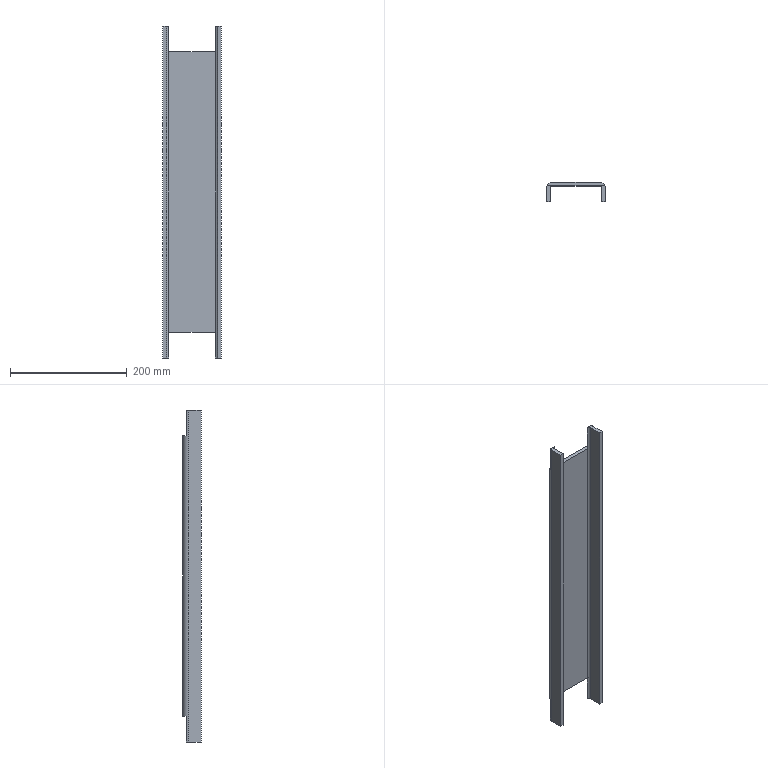Part | SolidWorks | features ICE 2, Extrusion 1 | 1 solid | 22 faces | box 100 x 32 x 568 mm | volume 448322 mm3 | plane 18 | cylinder 4 | commonest cylinder face diameters 8 x2 20 x2
STEP:
#1=CARTESIAN_POINT('',(90.,32.,524.));
#2=VERTEX_POINT('',#1);
#3=CARTESIAN_POINT('',(90.,32.,44.));
#4=VERTEX_POINT('',#3);
#5=CARTESIAN_POINT('',(90.,32.,568.));
#6=DIRECTION('',(0.,0.,-1.));
#7=VECTOR('',#6,1000.);
#8=LINE('',#5,#7);
#9=EDGE_CURVE('',#2,#4,#8,.T.);
#10=ORIENTED_EDGE('',*,*,#9,.T.);
#11=CARTESIAN_POINT('',(10.,32.,44.));
#12=VERTEX_POINT('',#11);
#13=CARTESIAN_POINT('',(10.,32.,44.));
#14=DIRECTION('',(-1.,0.,0.));
#15=VECTOR('',#14,1000.);
#16=LINE('',#13,#15);
#17=EDGE_CURVE('',#4,#12,#16,.T.);
#18=ORIENTED_EDGE('',*,*,#17,.T.);
#19=CARTESIAN_POINT('',(10.,32.,524.));
#20=VERTEX_POINT('',#19);
#21=CARTESIAN_POINT('',(10.,32.,568.));
#22=DIRECTION('',(0.,0.,-1.));
#23=VECTOR('',#22,1000.);
#24=LINE('',#21,#23);
#25=EDGE_CURVE('',#20,#12,#24,.T.);
#26=ORIENTED_EDGE('',*,*,#25,.F.);
#27=CARTESIAN_POINT('',(10.,32.,524.));
#28=DIRECTION('',(1.,0.,0.));
#29=VECTOR('',#28,1000.);
#30=LINE('',#27,#29);
#31=EDGE_CURVE('',#20,#2,#30,.T.);
#32=ORIENTED_EDGE('',*,*,#31,.T.);
#33=EDGE_LOOP('',(#10,#18,#26,#32));
#34=FACE_OUTER_BOUND('',#33,.T.);
#35=CARTESIAN_POINT('',(10.,32.,568.));
#36=DIRECTION('',(0.,1.,0.));
#37=DIRECTION('',(0.,0.,1.));
#38=AXIS2_PLACEMENT_3D('',#35,#36,#37);
#39=PLANE('',#38);
#40=ADVANCED_FACE('',(#34),#39,.T.);
#41=CARTESIAN_POINT('',(90.,26.,44.));
#42=VERTEX_POINT('',#41);
#43=CARTESIAN_POINT('',(10.,26.,44.));
#44=VERTEX_POINT('',#43);
#45=CARTESIAN_POINT('',(112.02,26.,44.));
#46=DIRECTION('',(-1.,0.,0.));
#47=VECTOR('',#46,1000.);
#48=LINE('',#45,#47);
#49=EDGE_CURVE('',#42,#44,#48,.T.);
#50=ORIENTED_EDGE('',*,*,#49,.F.);
#51=CARTESIAN_POINT('',(90.,26.,524.));
#52=VERTEX_POINT('',#51);
#53=CARTESIAN_POINT('',(90.,26.,568.));
#54=DIRECTION('',(0.,0.,-1.));
#55=VECTOR('',#54,1000.);
#56=LINE('',#53,#55);
#57=EDGE_CURVE('',#52,#42,#56,.T.);
#58=ORIENTED_EDGE('',*,*,#57,.F.);
#59=CARTESIAN_POINT('',(10.,26.,524.));
#60=VERTEX_POINT('',#59);
#61=CARTESIAN_POINT('',(-5.017,26.,524.));
#62=DIRECTION('',(1.,0.,0.));
#63=VECTOR('',#62,1000.);
#64=LINE('',#61,#63);
#65=EDGE_CURVE('',#60,#52,#64,.T.);
#66=ORIENTED_EDGE('',*,*,#65,.F.);
#67=CARTESIAN_POINT('',(10.,26.,568.));
#68=DIRECTION('',(0.,0.,-1.));
#69=VECTOR('',#68,1000.);
#70=LINE('',#67,#69);
#71=EDGE_CURVE('',#60,#44,#70,.T.);
#72=ORIENTED_EDGE('',*,*,#71,.T.);
#73=EDGE_LOOP('',(#50,#58,#66,#72));
#74=FACE_OUTER_BOUND('',#73,.T.);
#75=CARTESIAN_POINT('',(10.,26.,568.));
#76=DIRECTION('',(0.,1.,0.));
#77=DIRECTION('',(0.,0.,1.));
#78=AXIS2_PLACEMENT_3D('',#75,#76,#77);
#79=PLANE('',#78);
#80=ADVANCED_FACE('',(#74),#79,.F.);
#81=CARTESIAN_POINT('',(99.165,26.,0.));
#82=VERTEX_POINT('',#81);
#83=CARTESIAN_POINT('',(90.,26.,0.));
#84=VERTEX_POINT('',#83);
#85=CARTESIAN_POINT('',(90.,26.,0.));
#86=DIRECTION('',(-1.,0.,0.));
#87=VECTOR('',#86,1000.);
#88=LINE('',#85,#87);
#89=EDGE_CURVE('',#82,#84,#88,.T.);
#90=ORIENTED_EDGE('',*,*,#89,.F.);
#91=CARTESIAN_POINT('',(100.,22.,0.));
#92=VERTEX_POINT('',#91);
#93=CARTESIAN_POINT('',(90.,22.,0.));
#94=DIRECTION('',(0.,0.,-1.));
#95=DIRECTION('',(-1.,0.,0.));
#96=AXIS2_PLACEMENT_3D('',#93,#94,#95);
#97=CIRCLE('',#96,10.);
#98=EDGE_CURVE('',#82,#92,#97,.T.);
#99=ORIENTED_EDGE('',*,*,#98,.T.);
#100=CARTESIAN_POINT('',(100.,0.,0.));
#101=VERTEX_POINT('',#100);
#102=CARTESIAN_POINT('',(100.,22.,0.));
#103=DIRECTION('',(0.,-1.,0.));
#104=VECTOR('',#103,1000.);
#105=LINE('',#102,#104);
#106=EDGE_CURVE('',#92,#101,#105,.T.);
#107=ORIENTED_EDGE('',*,*,#106,.T.);
#108=CARTESIAN_POINT('',(94.,0.,0.));
#109=VERTEX_POINT('',#108);
#110=CARTESIAN_POINT('',(94.,0.,0.));
#111=DIRECTION('',(1.,0.,0.));
#112=VECTOR('',#111,1000.);
#113=LINE('',#110,#112);
#114=EDGE_CURVE('',#109,#101,#113,.T.);
#115=ORIENTED_EDGE('',*,*,#114,.F.);
#116=CARTESIAN_POINT('',(94.,22.,0.));
#117=VERTEX_POINT('',#116);
#118=CARTESIAN_POINT('',(94.,22.,0.));
#119=DIRECTION('',(0.,-1.,0.));
#120=VECTOR('',#119,1000.);
#121=LINE('',#118,#120);
#122=EDGE_CURVE('',#117,#109,#121,.T.);
#123=ORIENTED_EDGE('',*,*,#122,.F.);
#124=CARTESIAN_POINT('',(90.,22.,0.));
#125=DIRECTION('',(0.,0.,-1.));
#126=DIRECTION('',(-1.,0.,0.));
#127=AXIS2_PLACEMENT_3D('',#124,#125,#126);
#128=CIRCLE('',#127,4.);
#129=EDGE_CURVE('',#84,#117,#128,.T.);
#130=ORIENTED_EDGE('',*,*,#129,.F.);
#131=EDGE_LOOP('',(#90,#99,#107,#115,#123,#130));
#132=FACE_OUTER_BOUND('',#131,.T.);
#133=CARTESIAN_POINT('',(90.,22.,0.));
#134=DIRECTION('',(0.,0.,-1.));
#135=DIRECTION('',(-1.,0.,0.));
#136=AXIS2_PLACEMENT_3D('',#133,#134,#135);
#137=PLANE('',#136);
#138=ADVANCED_FACE('',(#132),#137,.T.);
#139=CARTESIAN_POINT('',(99.165,26.,568.));
#140=VERTEX_POINT('',#139);
#141=CARTESIAN_POINT('',(100.,22.,568.));
#142=VERTEX_POINT('',#141);
#143=CARTESIAN_POINT('',(90.,22.,568.));
#144=DIRECTION('',(0.,0.,-1.));
#145=DIRECTION('',(-1.,0.,0.));
#146=AXIS2_PLACEMENT_3D('',#143,#144,#145);
#147=CIRCLE('',#146,10.);
#148=EDGE_CURVE('',#140,#142,#147,.T.);
#149=ORIENTED_EDGE('',*,*,#148,.F.);
#150=CARTESIAN_POINT('',(90.,26.,568.));
#151=VERTEX_POINT('',#150);
#152=CARTESIAN_POINT('',(90.,26.,568.));
#153=DIRECTION('',(-1.,0.,0.));
#154=VECTOR('',#153,1000.);
#155=LINE('',#152,#154);
#156=EDGE_CURVE('',#140,#151,#155,.T.);
#157=ORIENTED_EDGE('',*,*,#156,.T.);
#158=CARTESIAN_POINT('',(94.,22.,568.));
#159=VERTEX_POINT('',#158);
#160=CARTESIAN_POINT('',(90.,22.,568.));
#161=DIRECTION('',(0.,0.,-1.));
#162=DIRECTION('',(-1.,0.,0.));
#163=AXIS2_PLACEMENT_3D('',#160,#161,#162);
#164=CIRCLE('',#163,4.);
#165=EDGE_CURVE('',#151,#159,#164,.T.);
#166=ORIENTED_EDGE('',*,*,#165,.T.);
#167=CARTESIAN_POINT('',(94.,0.,568.));
#168=VERTEX_POINT('',#167);
#169=CARTESIAN_POINT('',(94.,22.,568.));
#170=DIRECTION('',(0.,-1.,0.));
#171=VECTOR('',#170,1000.);
#172=LINE('',#169,#171);
#173=EDGE_CURVE('',#159,#168,#172,.T.);
#174=ORIENTED_EDGE('',*,*,#173,.T.);
#175=CARTESIAN_POINT('',(100.,0.,568.));
#176=VERTEX_POINT('',#175);
#177=CARTESIAN_POINT('',(94.,0.,568.));
#178=DIRECTION('',(1.,0.,0.));
#179=VECTOR('',#178,1000.);
#180=LINE('',#177,#179);
#181=EDGE_CURVE('',#168,#176,#180,.T.);
#182=ORIENTED_EDGE('',*,*,#181,.T.);
#183=CARTESIAN_POINT('',(100.,22.,568.));
#184=DIRECTION('',(0.,-1.,0.));
#185=VECTOR('',#184,1000.);
#186=LINE('',#183,#185);
#187=EDGE_CURVE('',#142,#176,#186,.T.);
#188=ORIENTED_EDGE('',*,*,#187,.F.);
#189=EDGE_LOOP('',(#149,#157,#166,#174,#182,#188));
#190=FACE_OUTER_BOUND('',#189,.T.);
#191=CARTESIAN_POINT('',(90.,22.,568.));
#192=DIRECTION('',(0.,0.,-1.));
#193=DIRECTION('',(-1.,0.,0.));
#194=AXIS2_PLACEMENT_3D('',#191,#192,#193);
#195=PLANE('',#194);
#196=ADVANCED_FACE('',(#190),#195,.F.);
#197=ORIENTED_EDGE('',*,*,#122,.T.);
#198=CARTESIAN_POINT('',(94.,0.,568.));
#199=DIRECTION('',(0.,0.,-1.));
#200=VECTOR('',#199,1000.);
#201=LINE('',#198,#200);
#202=EDGE_CURVE('',#168,#109,#201,.T.);
#203=ORIENTED_EDGE('',*,*,#202,.F.);
#204=ORIENTED_EDGE('',*,*,#173,.F.);
#205=CARTESIAN_POINT('',(94.,22.,568.));
#206=DIRECTION('',(0.,0.,-1.));
#207=VECTOR('',#206,1000.);
#208=LINE('',#205,#207);
#209=EDGE_CURVE('',#159,#117,#208,.T.);
#210=ORIENTED_EDGE('',*,*,#209,.T.);
#211=EDGE_LOOP('',(#197,#203,#204,#210));
#212=FACE_OUTER_BOUND('',#211,.T.);
#213=CARTESIAN_POINT('',(94.,22.,568.));
#214=DIRECTION('',(1.,0.,0.));
#215=DIRECTION('',(0.,0.,-1.));
#216=AXIS2_PLACEMENT_3D('',#213,#214,#215);
#217=PLANE('',#216);
#218=ADVANCED_FACE('',(#212),#217,.F.);
#219=ORIENTED_EDGE('',*,*,#114,.T.);
#220=CARTESIAN_POINT('',(100.,0.,568.));
#221=DIRECTION('',(0.,0.,-1.));
#222=VECTOR('',#221,1000.);
#223=LINE('',#220,#222);
#224=EDGE_CURVE('',#176,#101,#223,.T.);
#225=ORIENTED_EDGE('',*,*,#224,.F.);
#226=ORIENTED_EDGE('',*,*,#181,.F.);
#227=ORIENTED_EDGE('',*,*,#202,.T.);
#228=EDGE_LOOP('',(#219,#225,#226,#227));
#229=FACE_OUTER_BOUND('',#228,.T.);
#230=CARTESIAN_POINT('',(94.,0.,568.));
#231=DIRECTION('',(0.,1.,0.));
#232=DIRECTION('',(0.,0.,1.));
#233=AXIS2_PLACEMENT_3D('',#230,#231,#232);
#234=PLANE('',#233);
#235=ADVANCED_FACE('',(#229),#234,.F.);
#236=ORIENTED_EDGE('',*,*,#106,.F.);
#237=CARTESIAN_POINT('',(100.,22.,568.));
#238=DIRECTION('',(0.,0.,-1.));
#239=VECTOR('',#238,1000.);
#240=LINE('',#237,#239);
#241=EDGE_CURVE('',#142,#92,#240,.T.);
#242=ORIENTED_EDGE('',*,*,#241,.F.);
#243=ORIENTED_EDGE('',*,*,#187,.T.);
#244=ORIENTED_EDGE('',*,*,#224,.T.);
#245=EDGE_LOOP('',(#236,#242,#243,#244));
#246=FACE_OUTER_BOUND('',#245,.T.);
#247=CARTESIAN_POINT('',(100.,22.,568.));
#248=DIRECTION('',(1.,0.,0.));
#249=DIRECTION('',(0.,0.,-1.));
#250=AXIS2_PLACEMENT_3D('',#247,#248,#249);
#251=PLANE('',#250);
#252=ADVANCED_FACE('',(#246),#251,.T.);
#253=CARTESIAN_POINT('',(99.165,26.,44.));
#254=VERTEX_POINT('',#253);
#255=CARTESIAN_POINT('',(99.165,26.,568.));
#256=DIRECTION('',(0.,0.,-1.));
#257=VECTOR('',#256,1000.);
#258=LINE('',#255,#257);
#259=EDGE_CURVE('',#254,#82,#258,.T.);
#260=ORIENTED_EDGE('',*,*,#259,.F.);
#261=CARTESIAN_POINT('',(90.,22.,44.));
#262=DIRECTION('',(0.,0.,1.));
#263=DIRECTION('',(-1.,0.,0.));
#264=AXIS2_PLACEMENT_3D('',#261,#262,#263);
#265=CIRCLE('',#264,10.);
#266=EDGE_CURVE('',#254,#4,#265,.T.);
#267=ORIENTED_EDGE('',*,*,#266,.T.);
#268=ORIENTED_EDGE('',*,*,#9,.F.);
#269=CARTESIAN_POINT('',(99.165,26.,524.));
#270=VERTEX_POINT('',#269);
#271=CARTESIAN_POINT('',(90.,22.,524.));
#272=DIRECTION('',(0.,0.,-1.));
#273=DIRECTION('',(1.,0.,0.));
#274=AXIS2_PLACEMENT_3D('',#271,#272,#273);
#275=CIRCLE('',#274,10.);
#276=EDGE_CURVE('',#2,#270,#275,.T.);
#277=ORIENTED_EDGE('',*,*,#276,.T.);
#278=CARTESIAN_POINT('',(99.165,26.,568.));
#279=DIRECTION('',(0.,0.,-1.));
#280=VECTOR('',#279,1000.);
#281=LINE('',#278,#280);
#282=EDGE_CURVE('',#140,#270,#281,.T.);
#283=ORIENTED_EDGE('',*,*,#282,.F.);
#284=ORIENTED_EDGE('',*,*,#148,.T.);
#285=ORIENTED_EDGE('',*,*,#241,.T.);
#286=ORIENTED_EDGE('',*,*,#98,.F.);
#287=EDGE_LOOP('',(#260,#267,#268,#277,#283,#284,#285,#286));
#288=FACE_OUTER_BOUND('',#287,.T.);
#289=CARTESIAN_POINT('',(90.,22.,568.));
#290=DIRECTION('',(0.,0.,-1.));
#291=DIRECTION('',(-1.,0.,0.));
#292=AXIS2_PLACEMENT_3D('',#289,#290,#291);
#293=CYLINDRICAL_SURFACE('',#292,10.);
#294=ADVANCED_FACE('',(#288),#293,.T.);
#295=CARTESIAN_POINT('',(0.8348,26.,0.));
#296=VERTEX_POINT('',#295);
#297=CARTESIAN_POINT('',(0.8348,26.,44.));
#298=VERTEX_POINT('',#297);
#299=CARTESIAN_POINT('',(0.8348,26.,568.));
#300=DIRECTION('',(0.,0.,1.));
#301=VECTOR('',#300,1000.);
#302=LINE('',#299,#301);
#303=EDGE_CURVE('',#296,#298,#302,.T.);
#304=ORIENTED_EDGE('',*,*,#303,.F.);
#305=CARTESIAN_POINT('',(0.,22.,0.));
#306=VERTEX_POINT('',#305);
#307=CARTESIAN_POINT('',(10.,22.,0.));
#308=DIRECTION('',(0.,0.,-1.));
#309=DIRECTION('',(-1.,0.,0.));
#310=AXIS2_PLACEMENT_3D('',#307,#308,#309);
#311=CIRCLE('',#310,10.);
#312=EDGE_CURVE('',#306,#296,#311,.T.);
#313=ORIENTED_EDGE('',*,*,#312,.F.);
#314=CARTESIAN_POINT('',(0.,22.,568.));
#315=VERTEX_POINT('',#314);
#316=CARTESIAN_POINT('',(0.,22.,568.));
#317=DIRECTION('',(0.,0.,-1.));
#318=VECTOR('',#317,1000.);
#319=LINE('',#316,#318);
#320=EDGE_CURVE('',#315,#306,#319,.T.);
#321=ORIENTED_EDGE('',*,*,#320,.F.);
#322=CARTESIAN_POINT('',(0.8348,26.,568.));
#323=VERTEX_POINT('',#322);
#324=CARTESIAN_POINT('',(10.,22.,568.));
#325=DIRECTION('',(0.,0.,-1.));
#326=DIRECTION('',(-1.,0.,0.));
#327=AXIS2_PLACEMENT_3D('',#324,#325,#326);
#328=CIRCLE('',#327,10.);
#329=EDGE_CURVE('',#315,#323,#328,.T.);
#330=ORIENTED_EDGE('',*,*,#329,.T.);
#331=CARTESIAN_POINT('',(0.8348,26.,524.));
#332=VERTEX_POINT('',#331);
#333=CARTESIAN_POINT('',(0.8348,26.,568.));
#334=DIRECTION('',(0.,0.,1.));
#335=VECTOR('',#334,1000.);
#336=LINE('',#333,#335);
#337=EDGE_CURVE('',#332,#323,#336,.T.);
#338=ORIENTED_EDGE('',*,*,#337,.F.);
#339=CARTESIAN_POINT('',(10.,22.,524.));
#340=DIRECTION('',(0.,0.,-1.));
#341=DIRECTION('',(1.,0.,0.));
#342=AXIS2_PLACEMENT_3D('',#339,#340,#341);
#343=CIRCLE('',#342,10.);
#344=EDGE_CURVE('',#332,#20,#343,.T.);
#345=ORIENTED_EDGE('',*,*,#344,.T.);
#346=ORIENTED_EDGE('',*,*,#25,.T.);
#347=CARTESIAN_POINT('',(10.,22.,44.));
#348=DIRECTION('',(0.,0.,1.));
#349=DIRECTION('',(-1.,0.,0.));
#350=AXIS2_PLACEMENT_3D('',#347,#348,#349);
#351=CIRCLE('',#350,10.);
#352=EDGE_CURVE('',#12,#298,#351,.T.);
#353=ORIENTED_EDGE('',*,*,#352,.T.);
#354=EDGE_LOOP('',(#304,#313,#321,#330,#338,#345,#346,#353));
#355=FACE_OUTER_BOUND('',#354,.T.);
#356=CARTESIAN_POINT('',(10.,22.,568.));
#357=DIRECTION('',(0.,0.,-1.));
#358=DIRECTION('',(-1.,0.,0.));
#359=AXIS2_PLACEMENT_3D('',#356,#357,#358);
#360=CYLINDRICAL_SURFACE('',#359,10.);
#361=ADVANCED_FACE('',(#355),#360,.T.);
#362=CARTESIAN_POINT('',(0.,0.,0.));
#363=VERTEX_POINT('',#362);
#364=CARTESIAN_POINT('',(0.,0.,0.));
#365=DIRECTION('',(0.,1.,0.));
#366=VECTOR('',#365,1000.);
#367=LINE('',#364,#366);
#368=EDGE_CURVE('',#363,#306,#367,.T.);
#369=ORIENTED_EDGE('',*,*,#368,.F.);
#370=CARTESIAN_POINT('',(0.,0.,568.));
#371=VERTEX_POINT('',#370);
#372=CARTESIAN_POINT('',(0.,0.,568.));
#373=DIRECTION('',(0.,0.,-1.));
#374=VECTOR('',#373,1000.);
#375=LINE('',#372,#374);
#376=EDGE_CURVE('',#371,#363,#375,.T.);
#377=ORIENTED_EDGE('',*,*,#376,.F.);
#378=CARTESIAN_POINT('',(0.,0.,568.));
#379=DIRECTION('',(0.,1.,0.));
#380=VECTOR('',#379,1000.);
#381=LINE('',#378,#380);
#382=EDGE_CURVE('',#371,#315,#381,.T.);
#383=ORIENTED_EDGE('',*,*,#382,.T.);
#384=ORIENTED_EDGE('',*,*,#320,.T.);
#385=EDGE_LOOP('',(#369,#377,#383,#384));
#386=FACE_OUTER_BOUND('',#385,.T.);
#387=CARTESIAN_POINT('',(0.,0.,568.));
#388=DIRECTION('',(-1.,0.,0.));
#389=DIRECTION('',(0.,0.,1.));
#390=AXIS2_PLACEMENT_3D('',#387,#388,#389);
#391=PLANE('',#390);
#392=ADVANCED_FACE('',(#386),#391,.T.);
#393=CARTESIAN_POINT('',(6.,0.,0.));
#394=VERTEX_POINT('',#393);
#395=CARTESIAN_POINT('',(6.,0.,0.));
#396=DIRECTION('',(-1.,0.,0.));
#397=VECTOR('',#396,1000.);
#398=LINE('',#395,#397);
#399=EDGE_CURVE('',#394,#363,#398,.T.);
#400=ORIENTED_EDGE('',*,*,#399,.F.);
#401=CARTESIAN_POINT('',(6.,0.,568.));
#402=VERTEX_POINT('',#401);
#403=CARTESIAN_POINT('',(6.,0.,568.));
#404=DIRECTION('',(0.,0.,-1.));
#405=VECTOR('',#404,1000.);
#406=LINE('',#403,#405);
#407=EDGE_CURVE('',#402,#394,#406,.T.);
#408=ORIENTED_EDGE('',*,*,#407,.F.);
#409=CARTESIAN_POINT('',(6.,0.,568.));
#410=DIRECTION('',(-1.,0.,0.));
#411=VECTOR('',#410,1000.);
#412=LINE('',#409,#411);
#413=EDGE_CURVE('',#402,#371,#412,.T.);
#414=ORIENTED_EDGE('',*,*,#413,.T.);
#415=ORIENTED_EDGE('',*,*,#376,.T.);
#416=EDGE_LOOP('',(#400,#408,#414,#415));
#417=FACE_OUTER_BOUND('',#416,.T.);
#418=CARTESIAN_POINT('',(6.,0.,568.));
#419=DIRECTION('',(0.,-1.,0.));
#420=DIRECTION('',(0.,0.,-1.));
#421=AXIS2_PLACEMENT_3D('',#418,#419,#420);
#422=PLANE('',#421);
#423=ADVANCED_FACE('',(#417),#422,.T.);
#424=CARTESIAN_POINT('',(6.,22.,0.));
#425=VERTEX_POINT('',#424);
#426=CARTESIAN_POINT('',(6.,0.,0.));
#427=DIRECTION('',(0.,1.,0.));
#428=VECTOR('',#427,1000.);
#429=LINE('',#426,#428);
#430=EDGE_CURVE('',#394,#425,#429,.T.);
#431=ORIENTED_EDGE('',*,*,#430,.T.);
#432=CARTESIAN_POINT('',(6.,22.,568.));
#433=VERTEX_POINT('',#432);
#434=CARTESIAN_POINT('',(6.,22.,568.));
#435=DIRECTION('',(0.,0.,-1.));
#436=VECTOR('',#435,1000.);
#437=LINE('',#434,#436);
#438=EDGE_CURVE('',#433,#425,#437,.T.);
#439=ORIENTED_EDGE('',*,*,#438,.F.);
#440=CARTESIAN_POINT('',(6.,0.,568.));
#441=DIRECTION('',(0.,1.,0.));
#442=VECTOR('',#441,1000.);
#443=LINE('',#440,#442);
#444=EDGE_CURVE('',#402,#433,#443,.T.);
#445=ORIENTED_EDGE('',*,*,#444,.F.);
#446=ORIENTED_EDGE('',*,*,#407,.T.);
#447=EDGE_LOOP('',(#431,#439,#445,#446));
#448=FACE_OUTER_BOUND('',#447,.T.);
#449=CARTESIAN_POINT('',(6.,0.,568.));
#450=DIRECTION('',(-1.,0.,0.));
#451=DIRECTION('',(0.,0.,1.));
#452=AXIS2_PLACEMENT_3D('',#449,#450,#451);
#453=PLANE('',#452);
#454=ADVANCED_FACE('',(#448),#453,.F.);
#455=CARTESIAN_POINT('',(10.,26.,0.));
#456=VERTEX_POINT('',#455);
#457=CARTESIAN_POINT('',(10.,22.,0.));
#458=DIRECTION('',(0.,0.,-1.));
#459=DIRECTION('',(-1.,0.,0.));
#460=AXIS2_PLACEMENT_3D('',#457,#458,#459);
#461=CIRCLE('',#460,4.);
#462=EDGE_CURVE('',#425,#456,#461,.T.);
#463=ORIENTED_EDGE('',*,*,#462,.T.);
#464=CARTESIAN_POINT('',(10.,26.,568.));
#465=DIRECTION('',(0.,0.,1.));
#466=VECTOR('',#465,1000.);
#467=LINE('',#464,#466);
#468=EDGE_CURVE('',#456,#44,#467,.T.);
#469=ORIENTED_EDGE('',*,*,#468,.T.);
#470=ORIENTED_EDGE('',*,*,#71,.F.);
#471=CARTESIAN_POINT('',(10.,26.,568.));
#472=VERTEX_POINT('',#471);
#473=CARTESIAN_POINT('',(10.,26.,568.));
#474=DIRECTION('',(0.,0.,-1.));
#475=VECTOR('',#474,1000.);
#476=LINE('',#473,#475);
#477=EDGE_CURVE('',#472,#60,#476,.T.);
#478=ORIENTED_EDGE('',*,*,#477,.F.);
#479=CARTESIAN_POINT('',(10.,22.,568.));
#480=DIRECTION('',(0.,0.,-1.));
#481=DIRECTION('',(-1.,0.,0.));
#482=AXIS2_PLACEMENT_3D('',#479,#480,#481);
#483=CIRCLE('',#482,4.);
#484=EDGE_CURVE('',#433,#472,#483,.T.);
#485=ORIENTED_EDGE('',*,*,#484,.F.);
#486=ORIENTED_EDGE('',*,*,#438,.T.);
#487=EDGE_LOOP('',(#463,#469,#470,#478,#485,#486));
#488=FACE_OUTER_BOUND('',#487,.T.);
#489=CARTESIAN_POINT('',(10.,22.,568.));
#490=DIRECTION('',(0.,0.,-1.));
#491=DIRECTION('',(-1.,0.,0.));
#492=AXIS2_PLACEMENT_3D('',#489,#490,#491);
#493=CYLINDRICAL_SURFACE('',#492,4.);
#494=ADVANCED_FACE('',(#488),#493,.F.);
#495=ORIENTED_EDGE('',*,*,#129,.T.);
#496=ORIENTED_EDGE('',*,*,#209,.F.);
#497=ORIENTED_EDGE('',*,*,#165,.F.);
#498=CARTESIAN_POINT('',(90.,26.,568.));
#499=DIRECTION('',(0.,0.,-1.));
#500=VECTOR('',#499,1000.);
#501=LINE('',#498,#500);
#502=EDGE_CURVE('',#151,#52,#501,.T.);
#503=ORIENTED_EDGE('',*,*,#502,.T.);
#504=ORIENTED_EDGE('',*,*,#57,.T.);
#505=CARTESIAN_POINT('',(90.,26.,568.));
#506=DIRECTION('',(0.,0.,1.));
#507=VECTOR('',#506,1000.);
#508=LINE('',#505,#507);
#509=EDGE_CURVE('',#84,#42,#508,.T.);
#510=ORIENTED_EDGE('',*,*,#509,.F.);
#511=EDGE_LOOP('',(#495,#496,#497,#503,#504,#510));
#512=FACE_OUTER_BOUND('',#511,.T.);
#513=CARTESIAN_POINT('',(90.,22.,568.));
#514=DIRECTION('',(0.,0.,-1.));
#515=DIRECTION('',(-1.,0.,0.));
#516=AXIS2_PLACEMENT_3D('',#513,#514,#515);
#517=CYLINDRICAL_SURFACE('',#516,4.);
#518=ADVANCED_FACE('',(#512),#517,.F.);
#519=ORIENTED_EDGE('',*,*,#484,.T.);
#520=CARTESIAN_POINT('',(90.,26.,568.));
#521=DIRECTION('',(-1.,0.,0.));
#522=VECTOR('',#521,1000.);
#523=LINE('',#520,#522);
#524=EDGE_CURVE('',#472,#323,#523,.T.);
#525=ORIENTED_EDGE('',*,*,#524,.T.);
#526=ORIENTED_EDGE('',*,*,#329,.F.);
#527=ORIENTED_EDGE('',*,*,#382,.F.);
#528=ORIENTED_EDGE('',*,*,#413,.F.);
#529=ORIENTED_EDGE('',*,*,#444,.T.);
#530=EDGE_LOOP('',(#519,#525,#526,#527,#528,#529));
#531=FACE_OUTER_BOUND('',#530,.T.);
#532=CARTESIAN_POINT('',(90.,22.,568.));
#533=DIRECTION('',(0.,0.,-1.));
#534=DIRECTION('',(-1.,0.,0.));
#535=AXIS2_PLACEMENT_3D('',#532,#533,#534);
#536=PLANE('',#535);
#537=ADVANCED_FACE('',(#531),#536,.F.);
#538=CARTESIAN_POINT('',(90.,26.,0.));
#539=DIRECTION('',(-1.,0.,0.));
#540=VECTOR('',#539,1000.);
#541=LINE('',#538,#540);
#542=EDGE_CURVE('',#456,#296,#541,.T.);
#543=ORIENTED_EDGE('',*,*,#542,.F.);
#544=ORIENTED_EDGE('',*,*,#462,.F.);
#545=ORIENTED_EDGE('',*,*,#430,.F.);
#546=ORIENTED_EDGE('',*,*,#399,.T.);
#547=ORIENTED_EDGE('',*,*,#368,.T.);
#548=ORIENTED_EDGE('',*,*,#312,.T.);
#549=EDGE_LOOP('',(#543,#544,#545,#546,#547,#548));
#550=FACE_OUTER_BOUND('',#549,.T.);
#551=CARTESIAN_POINT('',(90.,22.,0.));
#552=DIRECTION('',(0.,0.,-1.));
#553=DIRECTION('',(-1.,0.,0.));
#554=AXIS2_PLACEMENT_3D('',#551,#552,#553);
#555=PLANE('',#554);
#556=ADVANCED_FACE('',(#550),#555,.T.);
#557=ORIENTED_EDGE('',*,*,#337,.T.);
#558=ORIENTED_EDGE('',*,*,#524,.F.);
#559=ORIENTED_EDGE('',*,*,#477,.T.);
#560=CARTESIAN_POINT('',(-5.017,26.,524.));
#561=DIRECTION('',(1.,0.,0.));
#562=VECTOR('',#561,1000.);
#563=LINE('',#560,#562);
#564=EDGE_CURVE('',#332,#60,#563,.T.);
#565=ORIENTED_EDGE('',*,*,#564,.F.);
#566=EDGE_LOOP('',(#557,#558,#559,#565));
#567=FACE_OUTER_BOUND('',#566,.T.);
#568=CARTESIAN_POINT('',(-5.017,26.,524.));
#569=DIRECTION('',(0.,-1.,0.));
#570=DIRECTION('',(0.,0.,-1.));
#571=AXIS2_PLACEMENT_3D('',#568,#569,#570);
#572=PLANE('',#571);
#573=ADVANCED_FACE('',(#567),#572,.F.);
#574=ORIENTED_EDGE('',*,*,#282,.T.);
#575=CARTESIAN_POINT('',(-5.017,26.,524.));
#576=DIRECTION('',(1.,0.,0.));
#577=VECTOR('',#576,1000.);
#578=LINE('',#575,#577);
#579=EDGE_CURVE('',#52,#270,#578,.T.);
#580=ORIENTED_EDGE('',*,*,#579,.F.);
#581=ORIENTED_EDGE('',*,*,#502,.F.);
#582=ORIENTED_EDGE('',*,*,#156,.F.);
#583=EDGE_LOOP('',(#574,#580,#581,#582));
#584=FACE_OUTER_BOUND('',#583,.T.);
#585=CARTESIAN_POINT('',(-5.017,26.,524.));
#586=DIRECTION('',(0.,-1.,0.));
#587=DIRECTION('',(0.,0.,-1.));
#588=AXIS2_PLACEMENT_3D('',#585,#586,#587);
#589=PLANE('',#588);
#590=ADVANCED_FACE('',(#584),#589,.F.);
#591=ORIENTED_EDGE('',*,*,#31,.F.);
#592=ORIENTED_EDGE('',*,*,#344,.F.);
#593=ORIENTED_EDGE('',*,*,#564,.T.);
#594=ORIENTED_EDGE('',*,*,#65,.T.);
#595=ORIENTED_EDGE('',*,*,#579,.T.);
#596=ORIENTED_EDGE('',*,*,#276,.F.);
#597=EDGE_LOOP('',(#591,#592,#593,#594,#595,#596));
#598=FACE_OUTER_BOUND('',#597,.T.);
#599=CARTESIAN_POINT('',(0.,0.,524.));
#600=DIRECTION('',(0.,0.,1.));
#601=DIRECTION('',(1.,0.,0.));
#602=AXIS2_PLACEMENT_3D('',#599,#600,#601);
#603=PLANE('',#602);
#604=ADVANCED_FACE('',(#598),#603,.T.);
#605=ORIENTED_EDGE('',*,*,#303,.T.);
#606=CARTESIAN_POINT('',(112.02,26.,44.));
#607=DIRECTION('',(-1.,0.,0.));
#608=VECTOR('',#607,1000.);
#609=LINE('',#606,#608);
#610=EDGE_CURVE('',#44,#298,#609,.T.);
#611=ORIENTED_EDGE('',*,*,#610,.F.);
#612=ORIENTED_EDGE('',*,*,#468,.F.);
#613=ORIENTED_EDGE('',*,*,#542,.T.);
#614=EDGE_LOOP('',(#605,#611,#612,#613));
#615=FACE_OUTER_BOUND('',#614,.T.);
#616=CARTESIAN_POINT('',(112.02,26.,44.));
#617=DIRECTION('',(0.,-1.,0.));
#618=DIRECTION('',(0.,0.,-1.));
#619=AXIS2_PLACEMENT_3D('',#616,#617,#618);
#620=PLANE('',#619);
#621=ADVANCED_FACE('',(#615),#620,.F.);
#622=ORIENTED_EDGE('',*,*,#259,.T.);
#623=ORIENTED_EDGE('',*,*,#89,.T.);
#624=ORIENTED_EDGE('',*,*,#509,.T.);
#625=CARTESIAN_POINT('',(112.02,26.,44.));
#626=DIRECTION('',(-1.,0.,0.));
#627=VECTOR('',#626,1000.);
#628=LINE('',#625,#627);
#629=EDGE_CURVE('',#254,#42,#628,.T.);
#630=ORIENTED_EDGE('',*,*,#629,.F.);
#631=EDGE_LOOP('',(#622,#623,#624,#630));
#632=FACE_OUTER_BOUND('',#631,.T.);
#633=CARTESIAN_POINT('',(112.02,26.,44.));
#634=DIRECTION('',(0.,-1.,0.));
#635=DIRECTION('',(0.,0.,-1.));
#636=AXIS2_PLACEMENT_3D('',#633,#634,#635);
#637=PLANE('',#636);
#638=ADVANCED_FACE('',(#632),#637,.F.);
#639=ORIENTED_EDGE('',*,*,#629,.T.);
#640=ORIENTED_EDGE('',*,*,#49,.T.);
#641=ORIENTED_EDGE('',*,*,#610,.T.);
#642=ORIENTED_EDGE('',*,*,#352,.F.);
#643=ORIENTED_EDGE('',*,*,#17,.F.);
#644=ORIENTED_EDGE('',*,*,#266,.F.);
#645=EDGE_LOOP('',(#639,#640,#641,#642,#643,#644));
#646=FACE_OUTER_BOUND('',#645,.T.);
#647=CARTESIAN_POINT('',(0.,0.,44.));
#648=DIRECTION('',(0.,0.,-1.));
#649=DIRECTION('',(-1.,0.,0.));
#650=AXIS2_PLACEMENT_3D('',#647,#648,#649);
#651=PLANE('',#650);
#652=ADVANCED_FACE('',(#646),#651,.T.);
#653=CLOSED_SHELL('',(#40,#80,#138,#196,#218,#235,#252,#294,#361,#392,#423,#454,#494,#518,#537,#556,#573,#590,#604,#621,#638,#652));
#654=MANIFOLD_SOLID_BREP('',#653);
#655=CARTESIAN_POINT('',(0.,0.,0.));
#656=DIRECTION('',(0.,0.,1.));
#657=DIRECTION('',(1.,0.,0.));
#658=AXIS2_PLACEMENT_3D('',#655,#656,#657);
#659=(LENGTH_UNIT()NAMED_UNIT(*)SI_UNIT(.MILLI.,.METRE.));
#660=UNCERTAINTY_MEASURE_WITH_UNIT(LENGTH_MEASURE(0.00001),#659,'','');
#661=(NAMED_UNIT(*)PLANE_ANGLE_UNIT()SI_UNIT($,.RADIAN.));
#662=(NAMED_UNIT(*)SI_UNIT($,.STERADIAN.)SOLID_ANGLE_UNIT());
#663=(GEOMETRIC_REPRESENTATION_CONTEXT(3)GLOBAL_UNCERTAINTY_ASSIGNED_CONTEXT((#660))GLOBAL_UNIT_ASSIGNED_CONTEXT((#659,#661,#662))REPRESENTATION_CONTEXT('',''));
#664=ADVANCED_BREP_SHAPE_REPRESENTATION('',(#654,#658),#663);